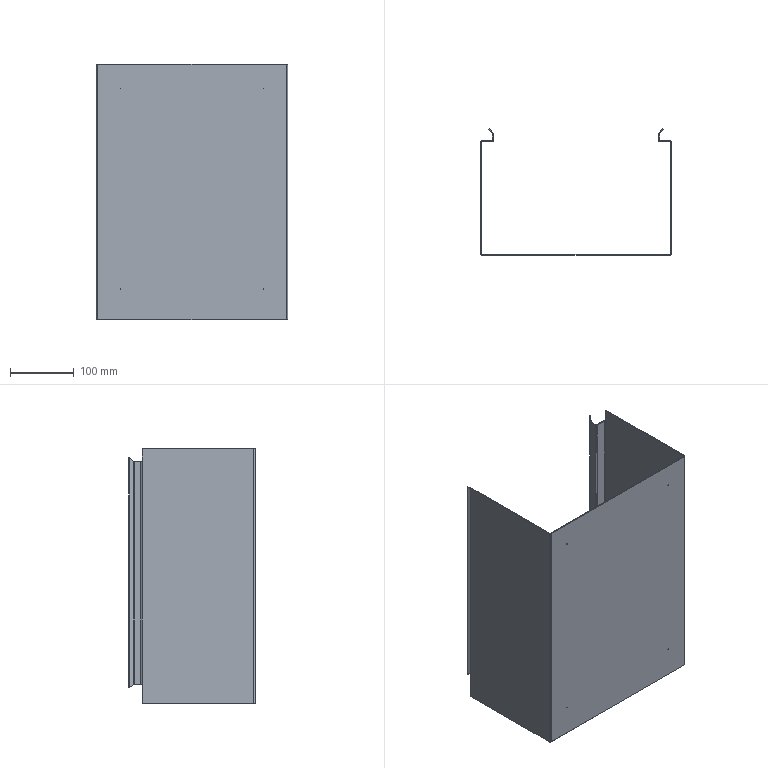Part | SolidWorks | features Cut 3, FlatPattern 1, SMBaseFlange 1, SheetMetal 1 | 1 solid | 86 faces | box 300 x 197.771 x 400 mm | volume 345884 mm3 | plane 62 | cylinder 24 | commonest cylinder face diameters 1 x8 2 x8 4.4 x8